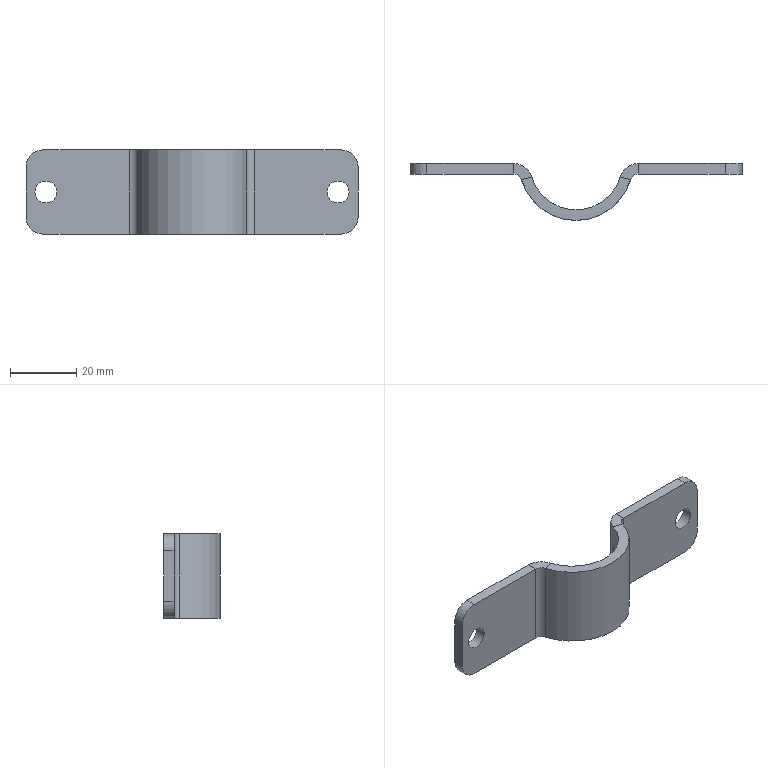Part | NX | features BREP 1 | 1 solid | 30 faces | box 100.076 x 17.145 x 25.4 mm | volume 8798 mm3 | plane 16 | cylinder 14 | commonest cylinder face diameters 6.604 x4 10.16 x4 4.978 x2 11.328 x2 27.94 x1 34.29 x1
STEP:
#1=CARTESIAN_POINT('',(-18.799,0.,12.7));
#2=VERTEX_POINT('',#1);
#3=CARTESIAN_POINT('',(-44.958,0.,12.7));
#4=VERTEX_POINT('',#3);
#5=CARTESIAN_POINT('',(-18.799,0.,12.7));
#6=DIRECTION('',(-1.,0.,0.));
#7=VECTOR('',#6,1000.);
#8=LINE('',#5,#7);
#9=EDGE_CURVE('',#2,#4,#8,.T.);
#10=ORIENTED_EDGE('',*,*,#9,.F.);
#11=CARTESIAN_POINT('',(-18.799,0.,-12.7));
#12=VERTEX_POINT('',#11);
#13=CARTESIAN_POINT('',(-18.799,0.,12.7));
#14=DIRECTION('',(0.,0.,-1.));
#15=VECTOR('',#14,1000.);
#16=LINE('',#13,#15);
#17=EDGE_CURVE('',#2,#12,#16,.T.);
#18=ORIENTED_EDGE('',*,*,#17,.T.);
#19=CARTESIAN_POINT('',(-44.958,0.,-12.7));
#20=VERTEX_POINT('',#19);
#21=CARTESIAN_POINT('',(-18.799,0.,-12.7));
#22=DIRECTION('',(-1.,0.,0.));
#23=VECTOR('',#22,1000.);
#24=LINE('',#21,#23);
#25=EDGE_CURVE('',#12,#20,#24,.T.);
#26=ORIENTED_EDGE('',*,*,#25,.T.);
#27=CARTESIAN_POINT('',(-50.038,0.,-7.62));
#28=VERTEX_POINT('',#27);
#29=CARTESIAN_POINT('',(-44.958,0.,-7.62));
#30=DIRECTION('',(0.,1.,0.));
#31=DIRECTION('',(0.,0.,-1.));
#32=AXIS2_PLACEMENT_3D('',#29,#30,#31);
#33=CIRCLE('',#32,5.08);
#34=EDGE_CURVE('',#20,#28,#33,.T.);
#35=ORIENTED_EDGE('',*,*,#34,.T.);
#36=CARTESIAN_POINT('',(-50.038,0.,7.62));
#37=VERTEX_POINT('',#36);
#38=CARTESIAN_POINT('',(-50.038,0.,7.62));
#39=DIRECTION('',(0.,0.,-1.));
#40=VECTOR('',#39,1000.);
#41=LINE('',#38,#40);
#42=EDGE_CURVE('',#37,#28,#41,.T.);
#43=ORIENTED_EDGE('',*,*,#42,.F.);
#44=CARTESIAN_POINT('',(-44.958,0.,7.62));
#45=DIRECTION('',(0.,1.,0.));
#46=DIRECTION('',(-1.,0.,0.));
#47=AXIS2_PLACEMENT_3D('',#44,#45,#46);
#48=CIRCLE('',#47,5.08);
#49=EDGE_CURVE('',#37,#4,#48,.T.);
#50=ORIENTED_EDGE('',*,*,#49,.T.);
#51=EDGE_LOOP('',(#10,#18,#26,#35,#43,#50));
#52=FACE_BOUND('',#51,.T.);
#53=CARTESIAN_POINT('',(-47.346,0.,0.));
#54=VERTEX_POINT('',#53);
#55=CARTESIAN_POINT('',(-40.742,0.,0.));
#56=VERTEX_POINT('',#55);
#57=CARTESIAN_POINT('',(-44.044,0.,0.));
#58=DIRECTION('',(0.,-1.,0.));
#59=DIRECTION('',(-1.,0.,0.));
#60=AXIS2_PLACEMENT_3D('',#57,#58,#59);
#61=CIRCLE('',#60,3.302);
#62=EDGE_CURVE('',#54,#56,#61,.T.);
#63=ORIENTED_EDGE('',*,*,#62,.T.);
#64=CARTESIAN_POINT('',(-44.044,0.,0.));
#65=DIRECTION('',(0.,-1.,0.));
#66=DIRECTION('',(1.,0.,0.));
#67=AXIS2_PLACEMENT_3D('',#64,#65,#66);
#68=CIRCLE('',#67,3.302);
#69=EDGE_CURVE('',#56,#54,#68,.T.);
#70=ORIENTED_EDGE('',*,*,#69,.T.);
#71=EDGE_LOOP('',(#63,#70));
#72=FACE_BOUND('',#71,.T.);
#73=CARTESIAN_POINT('',(-18.799,0.,12.7));
#74=DIRECTION('',(0.,1.,0.));
#75=DIRECTION('',(1.,0.,0.));
#76=AXIS2_PLACEMENT_3D('',#73,#74,#75);
#77=PLANE('',#76);
#78=ADVANCED_FACE('',(#52,#72),#77,.T.);
#79=CARTESIAN_POINT('',(-40.742,-3.175,0.));
#80=VERTEX_POINT('',#79);
#81=CARTESIAN_POINT('',(-40.742,0.,0.));
#82=DIRECTION('',(0.,-1.,0.));
#83=VECTOR('',#82,1000.);
#84=LINE('',#81,#83);
#85=EDGE_CURVE('',#80,#56,#84,.F.);
#86=ORIENTED_EDGE('',*,*,#85,.F.);
#87=CARTESIAN_POINT('',(-47.346,-3.175,0.));
#88=VERTEX_POINT('',#87);
#89=CARTESIAN_POINT('',(-44.044,-3.175,0.));
#90=DIRECTION('',(0.,-1.,0.));
#91=DIRECTION('',(1.,0.,0.));
#92=AXIS2_PLACEMENT_3D('',#89,#90,#91);
#93=CIRCLE('',#92,3.302);
#94=EDGE_CURVE('',#80,#88,#93,.T.);
#95=ORIENTED_EDGE('',*,*,#94,.T.);
#96=CARTESIAN_POINT('',(-47.346,0.,0.));
#97=DIRECTION('',(0.,-1.,0.));
#98=VECTOR('',#97,1000.);
#99=LINE('',#96,#98);
#100=EDGE_CURVE('',#88,#54,#99,.F.);
#101=ORIENTED_EDGE('',*,*,#100,.T.);
#102=ORIENTED_EDGE('',*,*,#69,.F.);
#103=EDGE_LOOP('',(#86,#95,#101,#102));
#104=FACE_BOUND('',#103,.T.);
#105=CARTESIAN_POINT('',(-44.044,-1.587,0.));
#106=DIRECTION('',(0.,-1.,0.));
#107=DIRECTION('',(1.,0.,0.));
#108=AXIS2_PLACEMENT_3D('',#105,#106,#107);
#109=CYLINDRICAL_SURFACE('',#108,3.302);
#110=ADVANCED_FACE('',(#104),#109,.F.);
#111=ORIENTED_EDGE('',*,*,#100,.F.);
#112=CARTESIAN_POINT('',(-44.044,-3.175,0.));
#113=DIRECTION('',(0.,-1.,0.));
#114=DIRECTION('',(-1.,0.,0.));
#115=AXIS2_PLACEMENT_3D('',#112,#113,#114);
#116=CIRCLE('',#115,3.302);
#117=EDGE_CURVE('',#88,#80,#116,.T.);
#118=ORIENTED_EDGE('',*,*,#117,.T.);
#119=ORIENTED_EDGE('',*,*,#85,.T.);
#120=ORIENTED_EDGE('',*,*,#62,.F.);
#121=EDGE_LOOP('',(#111,#118,#119,#120));
#122=FACE_BOUND('',#121,.T.);
#123=CARTESIAN_POINT('',(-44.044,-1.587,0.));
#124=DIRECTION('',(0.,-1.,0.));
#125=DIRECTION('',(-1.,0.,0.));
#126=AXIS2_PLACEMENT_3D('',#123,#124,#125);
#127=CYLINDRICAL_SURFACE('',#126,3.302);
#128=ADVANCED_FACE('',(#122),#127,.F.);
#129=CARTESIAN_POINT('',(-50.038,-3.175,7.62));
#130=VERTEX_POINT('',#129);
#131=CARTESIAN_POINT('',(-50.038,-3.175,-7.62));
#132=VERTEX_POINT('',#131);
#133=CARTESIAN_POINT('',(-50.038,-3.175,7.62));
#134=DIRECTION('',(0.,0.,-1.));
#135=VECTOR('',#134,1000.);
#136=LINE('',#133,#135);
#137=EDGE_CURVE('',#130,#132,#136,.T.);
#138=ORIENTED_EDGE('',*,*,#137,.T.);
#139=CARTESIAN_POINT('',(-44.958,-3.175,-12.7));
#140=VERTEX_POINT('',#139);
#141=CARTESIAN_POINT('',(-44.958,-3.175,-7.62));
#142=DIRECTION('',(0.,-1.,0.));
#143=DIRECTION('',(-1.,0.,0.));
#144=AXIS2_PLACEMENT_3D('',#141,#142,#143);
#145=CIRCLE('',#144,5.08);
#146=EDGE_CURVE('',#132,#140,#145,.T.);
#147=ORIENTED_EDGE('',*,*,#146,.T.);
#148=CARTESIAN_POINT('',(-18.799,-3.175,-12.7));
#149=VERTEX_POINT('',#148);
#150=CARTESIAN_POINT('',(-18.799,-3.175,-12.7));
#151=DIRECTION('',(-1.,0.,0.));
#152=VECTOR('',#151,1000.);
#153=LINE('',#150,#152);
#154=EDGE_CURVE('',#149,#140,#153,.T.);
#155=ORIENTED_EDGE('',*,*,#154,.F.);
#156=CARTESIAN_POINT('',(-18.799,-3.175,12.7));
#157=VERTEX_POINT('',#156);
#158=CARTESIAN_POINT('',(-18.799,-3.175,12.7));
#159=DIRECTION('',(0.,0.,-1.));
#160=VECTOR('',#159,1000.);
#161=LINE('',#158,#160);
#162=EDGE_CURVE('',#157,#149,#161,.T.);
#163=ORIENTED_EDGE('',*,*,#162,.F.);
#164=CARTESIAN_POINT('',(-44.958,-3.175,12.7));
#165=VERTEX_POINT('',#164);
#166=CARTESIAN_POINT('',(-18.799,-3.175,12.7));
#167=DIRECTION('',(-1.,0.,0.));
#168=VECTOR('',#167,1000.);
#169=LINE('',#166,#168);
#170=EDGE_CURVE('',#157,#165,#169,.T.);
#171=ORIENTED_EDGE('',*,*,#170,.T.);
#172=CARTESIAN_POINT('',(-44.958,-3.175,7.62));
#173=DIRECTION('',(0.,-1.,0.));
#174=DIRECTION('',(0.,0.,1.));
#175=AXIS2_PLACEMENT_3D('',#172,#173,#174);
#176=CIRCLE('',#175,5.08);
#177=EDGE_CURVE('',#165,#130,#176,.T.);
#178=ORIENTED_EDGE('',*,*,#177,.T.);
#179=EDGE_LOOP('',(#138,#147,#155,#163,#171,#178));
#180=FACE_BOUND('',#179,.T.);
#181=ORIENTED_EDGE('',*,*,#117,.F.);
#182=ORIENTED_EDGE('',*,*,#94,.F.);
#183=EDGE_LOOP('',(#181,#182));
#184=FACE_BOUND('',#183,.T.);
#185=CARTESIAN_POINT('',(-18.799,-3.175,12.7));
#186=DIRECTION('',(0.,1.,0.));
#187=DIRECTION('',(1.,0.,0.));
#188=AXIS2_PLACEMENT_3D('',#185,#186,#187);
#189=PLANE('',#188);
#190=ADVANCED_FACE('',(#180,#184),#189,.F.);
#191=ORIENTED_EDGE('',*,*,#177,.F.);
#192=CARTESIAN_POINT('',(-44.958,-3.175,12.7));
#193=DIRECTION('',(0.,1.,0.));
#194=VECTOR('',#193,1000.);
#195=LINE('',#192,#194);
#196=EDGE_CURVE('',#165,#4,#195,.T.);
#197=ORIENTED_EDGE('',*,*,#196,.T.);
#198=ORIENTED_EDGE('',*,*,#49,.F.);
#199=CARTESIAN_POINT('',(-50.038,-3.175,7.62));
#200=DIRECTION('',(0.,1.,0.));
#201=VECTOR('',#200,1000.);
#202=LINE('',#199,#201);
#203=EDGE_CURVE('',#130,#37,#202,.T.);
#204=ORIENTED_EDGE('',*,*,#203,.F.);
#205=EDGE_LOOP('',(#191,#197,#198,#204));
#206=FACE_BOUND('',#205,.T.);
#207=CARTESIAN_POINT('',(-44.958,-3.317,7.62));
#208=DIRECTION('',(0.,1.,0.));
#209=DIRECTION('',(-1.,0.,0.));
#210=AXIS2_PLACEMENT_3D('',#207,#208,#209);
#211=CYLINDRICAL_SURFACE('',#210,5.08);
#212=ADVANCED_FACE('',(#206),#211,.T.);
#213=ORIENTED_EDGE('',*,*,#42,.T.);
#214=CARTESIAN_POINT('',(-50.038,-3.175,-7.62));
#215=DIRECTION('',(0.,1.,0.));
#216=VECTOR('',#215,1000.);
#217=LINE('',#214,#216);
#218=EDGE_CURVE('',#132,#28,#217,.T.);
#219=ORIENTED_EDGE('',*,*,#218,.F.);
#220=ORIENTED_EDGE('',*,*,#137,.F.);
#221=ORIENTED_EDGE('',*,*,#203,.T.);
#222=EDGE_LOOP('',(#213,#219,#220,#221));
#223=FACE_BOUND('',#222,.T.);
#224=CARTESIAN_POINT('',(-50.038,-1.587,0.));
#225=DIRECTION('',(1.,0.,0.));
#226=DIRECTION('',(0.,1.,0.));
#227=AXIS2_PLACEMENT_3D('',#224,#225,#226);
#228=PLANE('',#227);
#229=ADVANCED_FACE('',(#223),#228,.F.);
#230=ORIENTED_EDGE('',*,*,#146,.F.);
#231=ORIENTED_EDGE('',*,*,#218,.T.);
#232=ORIENTED_EDGE('',*,*,#34,.F.);
#233=CARTESIAN_POINT('',(-44.958,-3.175,-12.7));
#234=DIRECTION('',(0.,1.,0.));
#235=VECTOR('',#234,1000.);
#236=LINE('',#233,#235);
#237=EDGE_CURVE('',#140,#20,#236,.T.);
#238=ORIENTED_EDGE('',*,*,#237,.F.);
#239=EDGE_LOOP('',(#230,#231,#232,#238));
#240=FACE_BOUND('',#239,.T.);
#241=CARTESIAN_POINT('',(-44.958,-3.317,-7.62));
#242=DIRECTION('',(0.,1.,0.));
#243=DIRECTION('',(0.,0.,-1.));
#244=AXIS2_PLACEMENT_3D('',#241,#242,#243);
#245=CYLINDRICAL_SURFACE('',#244,5.08);
#246=ADVANCED_FACE('',(#240),#245,.T.);
#247=ORIENTED_EDGE('',*,*,#25,.F.);
#248=CARTESIAN_POINT('',(-18.799,0.,-12.7));
#249=DIRECTION('',(0.,-1.,0.));
#250=VECTOR('',#249,1000.);
#251=LINE('',#248,#250);
#252=EDGE_CURVE('',#12,#149,#251,.T.);
#253=ORIENTED_EDGE('',*,*,#252,.T.);
#254=ORIENTED_EDGE('',*,*,#154,.T.);
#255=ORIENTED_EDGE('',*,*,#237,.T.);
#256=EDGE_LOOP('',(#247,#253,#254,#255));
#257=FACE_BOUND('',#256,.T.);
#258=CARTESIAN_POINT('',(-34.419,-1.587,-12.7));
#259=DIRECTION('',(0.,0.,-1.));
#260=DIRECTION('',(0.,-1.,0.));
#261=AXIS2_PLACEMENT_3D('',#258,#259,#260);
#262=PLANE('',#261);
#263=ADVANCED_FACE('',(#257),#262,.T.);
#264=CARTESIAN_POINT('',(-13.376,-4.03,-12.7));
#265=VERTEX_POINT('',#264);
#266=CARTESIAN_POINT('',(-16.416,-4.946,-12.7));
#267=VERTEX_POINT('',#266);
#268=CARTESIAN_POINT('',(-13.376,-4.03,-12.7));
#269=DIRECTION('',(-0.9575,-0.2885,0.));
#270=VECTOR('',#269,1000.);
#271=LINE('',#268,#270);
#272=EDGE_CURVE('',#265,#267,#271,.T.);
#273=ORIENTED_EDGE('',*,*,#272,.T.);
#274=CARTESIAN_POINT('',(-18.799,-5.664,-12.7));
#275=DIRECTION('',(0.,0.,1.));
#276=DIRECTION('',(0.9575,0.2885,0.));
#277=AXIS2_PLACEMENT_3D('',#274,#275,#276);
#278=CIRCLE('',#277,2.489);
#279=EDGE_CURVE('',#267,#149,#278,.T.);
#280=ORIENTED_EDGE('',*,*,#279,.T.);
#281=ORIENTED_EDGE('',*,*,#252,.F.);
#282=CARTESIAN_POINT('',(-18.799,-5.664,-12.7));
#283=DIRECTION('',(0.,0.,1.));
#284=DIRECTION('',(0.9575,0.2885,0.));
#285=AXIS2_PLACEMENT_3D('',#282,#283,#284);
#286=CIRCLE('',#285,5.664);
#287=EDGE_CURVE('',#265,#12,#286,.T.);
#288=ORIENTED_EDGE('',*,*,#287,.F.);
#289=EDGE_LOOP('',(#273,#280,#281,#288));
#290=FACE_BOUND('',#289,.T.);
#291=CARTESIAN_POINT('',(-16.368,-2.392,-12.7));
#292=DIRECTION('',(0.,0.,-1.));
#293=DIRECTION('',(0.,-1.,0.));
#294=AXIS2_PLACEMENT_3D('',#291,#292,#293);
#295=PLANE('',#294);
#296=ADVANCED_FACE('',(#290),#295,.T.);
#297=CARTESIAN_POINT('',(-13.376,-4.03,12.7));
#298=VERTEX_POINT('',#297);
#299=CARTESIAN_POINT('',(-13.376,-4.03,12.7));
#300=DIRECTION('',(0.,0.,-1.));
#301=VECTOR('',#300,1000.);
#302=LINE('',#299,#301);
#303=EDGE_CURVE('',#298,#265,#302,.T.);
#304=ORIENTED_EDGE('',*,*,#303,.T.);
#305=ORIENTED_EDGE('',*,*,#287,.T.);
#306=ORIENTED_EDGE('',*,*,#17,.F.);
#307=CARTESIAN_POINT('',(-18.799,-5.664,12.7));
#308=DIRECTION('',(0.,0.,1.));
#309=DIRECTION('',(0.9575,0.2885,0.));
#310=AXIS2_PLACEMENT_3D('',#307,#308,#309);
#311=CIRCLE('',#310,5.664);
#312=EDGE_CURVE('',#298,#2,#311,.T.);
#313=ORIENTED_EDGE('',*,*,#312,.F.);
#314=EDGE_LOOP('',(#304,#305,#306,#313));
#315=FACE_BOUND('',#314,.T.);
#316=CARTESIAN_POINT('',(-18.799,-5.664,12.7));
#317=DIRECTION('',(0.,0.,1.));
#318=DIRECTION('',(1.,0.,0.));
#319=AXIS2_PLACEMENT_3D('',#316,#317,#318);
#320=CYLINDRICAL_SURFACE('',#319,5.664);
#321=ADVANCED_FACE('',(#315),#320,.T.);
#322=CARTESIAN_POINT('',(-18.799,0.,12.7));
#323=DIRECTION('',(0.,-1.,0.));
#324=VECTOR('',#323,1000.);
#325=LINE('',#322,#324);
#326=EDGE_CURVE('',#2,#157,#325,.T.);
#327=ORIENTED_EDGE('',*,*,#326,.T.);
#328=CARTESIAN_POINT('',(-16.416,-4.946,12.7));
#329=VERTEX_POINT('',#328);
#330=CARTESIAN_POINT('',(-18.799,-5.664,12.7));
#331=DIRECTION('',(0.,0.,1.));
#332=DIRECTION('',(0.9575,0.2885,0.));
#333=AXIS2_PLACEMENT_3D('',#330,#331,#332);
#334=CIRCLE('',#333,2.489);
#335=EDGE_CURVE('',#329,#157,#334,.T.);
#336=ORIENTED_EDGE('',*,*,#335,.F.);
#337=CARTESIAN_POINT('',(-13.376,-4.03,12.7));
#338=DIRECTION('',(-0.9575,-0.2885,0.));
#339=VECTOR('',#338,1000.);
#340=LINE('',#337,#339);
#341=EDGE_CURVE('',#298,#329,#340,.T.);
#342=ORIENTED_EDGE('',*,*,#341,.F.);
#343=ORIENTED_EDGE('',*,*,#312,.T.);
#344=EDGE_LOOP('',(#327,#336,#342,#343));
#345=FACE_BOUND('',#344,.T.);
#346=CARTESIAN_POINT('',(-16.368,-2.392,12.7));
#347=DIRECTION('',(0.,0.,-1.));
#348=DIRECTION('',(0.,-1.,0.));
#349=AXIS2_PLACEMENT_3D('',#346,#347,#348);
#350=PLANE('',#349);
#351=ADVANCED_FACE('',(#345),#350,.F.);
#352=ORIENTED_EDGE('',*,*,#341,.T.);
#353=CARTESIAN_POINT('',(16.416,-4.946,12.7));
#354=VERTEX_POINT('',#353);
#355=CARTESIAN_POINT('',(0.,0.,12.7));
#356=DIRECTION('',(0.,0.,-1.));
#357=DIRECTION('',(0.9575,-0.2885,0.));
#358=AXIS2_PLACEMENT_3D('',#355,#356,#357);
#359=CIRCLE('',#358,17.145);
#360=EDGE_CURVE('',#354,#329,#359,.T.);
#361=ORIENTED_EDGE('',*,*,#360,.F.);
#362=CARTESIAN_POINT('',(13.376,-4.03,12.7));
#363=VERTEX_POINT('',#362);
#364=CARTESIAN_POINT('',(13.376,-4.03,12.7));
#365=DIRECTION('',(0.9575,-0.2885,0.));
#366=VECTOR('',#365,1000.);
#367=LINE('',#364,#366);
#368=EDGE_CURVE('',#363,#354,#367,.T.);
#369=ORIENTED_EDGE('',*,*,#368,.F.);
#370=CARTESIAN_POINT('',(0.,0.,12.7));
#371=DIRECTION('',(0.,0.,-1.));
#372=DIRECTION('',(0.9575,-0.2885,0.));
#373=AXIS2_PLACEMENT_3D('',#370,#371,#372);
#374=CIRCLE('',#373,13.97);
#375=EDGE_CURVE('',#363,#298,#374,.T.);
#376=ORIENTED_EDGE('',*,*,#375,.T.);
#377=EDGE_LOOP('',(#352,#361,#369,#376));
#378=FACE_BOUND('',#377,.T.);
#379=CARTESIAN_POINT('',(0.,-15.557,12.7));
#380=DIRECTION('',(0.,0.,-1.));
#381=DIRECTION('',(0.,-1.,0.));
#382=AXIS2_PLACEMENT_3D('',#379,#380,#381);
#383=PLANE('',#382);
#384=ADVANCED_FACE('',(#378),#383,.F.);
#385=CARTESIAN_POINT('',(13.376,-4.03,-12.7));
#386=VERTEX_POINT('',#385);
#387=CARTESIAN_POINT('',(13.376,-4.03,12.7));
#388=DIRECTION('',(0.,0.,-1.));
#389=VECTOR('',#388,1000.);
#390=LINE('',#387,#389);
#391=EDGE_CURVE('',#363,#386,#390,.T.);
#392=ORIENTED_EDGE('',*,*,#391,.T.);
#393=CARTESIAN_POINT('',(0.,0.,-12.7));
#394=DIRECTION('',(0.,0.,-1.));
#395=DIRECTION('',(0.9575,-0.2885,0.));
#396=AXIS2_PLACEMENT_3D('',#393,#394,#395);
#397=CIRCLE('',#396,13.97);
#398=EDGE_CURVE('',#386,#265,#397,.T.);
#399=ORIENTED_EDGE('',*,*,#398,.T.);
#400=ORIENTED_EDGE('',*,*,#303,.F.);
#401=ORIENTED_EDGE('',*,*,#375,.F.);
#402=EDGE_LOOP('',(#392,#399,#400,#401));
#403=FACE_BOUND('',#402,.T.);
#404=CARTESIAN_POINT('',(0.,0.,12.7));
#405=DIRECTION('',(0.,0.,1.));
#406=DIRECTION('',(1.,0.,0.));
#407=AXIS2_PLACEMENT_3D('',#404,#405,#406);
#408=CYLINDRICAL_SURFACE('',#407,13.97);
#409=ADVANCED_FACE('',(#403),#408,.F.);
#410=CARTESIAN_POINT('',(16.416,-4.946,-12.7));
#411=VERTEX_POINT('',#410);
#412=CARTESIAN_POINT('',(13.376,-4.03,-12.7));
#413=DIRECTION('',(0.9575,-0.2885,0.));
#414=VECTOR('',#413,1000.);
#415=LINE('',#412,#414);
#416=EDGE_CURVE('',#386,#411,#415,.T.);
#417=ORIENTED_EDGE('',*,*,#416,.T.);
#418=CARTESIAN_POINT('',(0.,0.,-12.7));
#419=DIRECTION('',(0.,0.,-1.));
#420=DIRECTION('',(0.9575,-0.2885,0.));
#421=AXIS2_PLACEMENT_3D('',#418,#419,#420);
#422=CIRCLE('',#421,17.145);
#423=EDGE_CURVE('',#411,#267,#422,.T.);
#424=ORIENTED_EDGE('',*,*,#423,.T.);
#425=ORIENTED_EDGE('',*,*,#272,.F.);
#426=ORIENTED_EDGE('',*,*,#398,.F.);
#427=EDGE_LOOP('',(#417,#424,#425,#426));
#428=FACE_BOUND('',#427,.T.);
#429=CARTESIAN_POINT('',(0.,-15.557,-12.7));
#430=DIRECTION('',(0.,0.,-1.));
#431=DIRECTION('',(0.,-1.,0.));
#432=AXIS2_PLACEMENT_3D('',#429,#430,#431);
#433=PLANE('',#432);
#434=ADVANCED_FACE('',(#428),#433,.T.);
#435=CARTESIAN_POINT('',(-16.416,-4.946,12.7));
#436=DIRECTION('',(0.,0.,-1.));
#437=VECTOR('',#436,1000.);
#438=LINE('',#435,#437);
#439=EDGE_CURVE('',#329,#267,#438,.T.);
#440=ORIENTED_EDGE('',*,*,#439,.T.);
#441=ORIENTED_EDGE('',*,*,#423,.F.);
#442=CARTESIAN_POINT('',(16.416,-4.946,12.7));
#443=DIRECTION('',(0.,0.,-1.));
#444=VECTOR('',#443,1000.);
#445=LINE('',#442,#444);
#446=EDGE_CURVE('',#354,#411,#445,.T.);
#447=ORIENTED_EDGE('',*,*,#446,.F.);
#448=ORIENTED_EDGE('',*,*,#360,.T.);
#449=EDGE_LOOP('',(#440,#441,#447,#448));
#450=FACE_BOUND('',#449,.T.);
#451=CARTESIAN_POINT('',(0.,0.,12.7));
#452=DIRECTION('',(0.,0.,1.));
#453=DIRECTION('',(1.,0.,0.));
#454=AXIS2_PLACEMENT_3D('',#451,#452,#453);
#455=CYLINDRICAL_SURFACE('',#454,17.145);
#456=ADVANCED_FACE('',(#450),#455,.T.);
#457=ORIENTED_EDGE('',*,*,#446,.T.);
#458=CARTESIAN_POINT('',(18.799,-3.175,-12.7));
#459=VERTEX_POINT('',#458);
#460=CARTESIAN_POINT('',(18.799,-5.664,-12.7));
#461=DIRECTION('',(0.,0.,1.));
#462=DIRECTION('',(0.,1.,0.));
#463=AXIS2_PLACEMENT_3D('',#460,#461,#462);
#464=CIRCLE('',#463,2.489);
#465=EDGE_CURVE('',#459,#411,#464,.T.);
#466=ORIENTED_EDGE('',*,*,#465,.F.);
#467=CARTESIAN_POINT('',(18.799,-3.175,12.7));
#468=VERTEX_POINT('',#467);
#469=CARTESIAN_POINT('',(18.799,-3.175,12.7));
#470=DIRECTION('',(0.,0.,-1.));
#471=VECTOR('',#470,1000.);
#472=LINE('',#469,#471);
#473=EDGE_CURVE('',#468,#459,#472,.T.);
#474=ORIENTED_EDGE('',*,*,#473,.F.);
#475=CARTESIAN_POINT('',(18.799,-5.664,12.7));
#476=DIRECTION('',(0.,0.,1.));
#477=DIRECTION('',(0.,1.,0.));
#478=AXIS2_PLACEMENT_3D('',#475,#476,#477);
#479=CIRCLE('',#478,2.489);
#480=EDGE_CURVE('',#468,#354,#479,.T.);
#481=ORIENTED_EDGE('',*,*,#480,.T.);
#482=EDGE_LOOP('',(#457,#466,#474,#481));
#483=FACE_BOUND('',#482,.T.);
#484=CARTESIAN_POINT('',(18.799,-5.664,12.7));
#485=DIRECTION('',(0.,0.,1.));
#486=DIRECTION('',(1.,0.,0.));
#487=AXIS2_PLACEMENT_3D('',#484,#485,#486);
#488=CYLINDRICAL_SURFACE('',#487,2.489);
#489=ADVANCED_FACE('',(#483),#488,.F.);
#490=ORIENTED_EDGE('',*,*,#368,.T.);
#491=ORIENTED_EDGE('',*,*,#480,.F.);
#492=CARTESIAN_POINT('',(18.799,0.,12.7));
#493=VERTEX_POINT('',#492);
#494=CARTESIAN_POINT('',(18.799,0.,12.7));
#495=DIRECTION('',(0.,-1.,0.));
#496=VECTOR('',#495,1000.);
#497=LINE('',#494,#496);
#498=EDGE_CURVE('',#493,#468,#497,.T.);
#499=ORIENTED_EDGE('',*,*,#498,.F.);
#500=CARTESIAN_POINT('',(18.799,-5.664,12.7));
#501=DIRECTION('',(0.,0.,1.));
#502=DIRECTION('',(0.,1.,0.));
#503=AXIS2_PLACEMENT_3D('',#500,#501,#502);
#504=CIRCLE('',#503,5.664);
#505=EDGE_CURVE('',#493,#363,#504,.T.);
#506=ORIENTED_EDGE('',*,*,#505,.T.);
#507=EDGE_LOOP('',(#490,#491,#499,#506));
#508=FACE_BOUND('',#507,.T.);
#509=CARTESIAN_POINT('',(16.368,-2.392,12.7));
#510=DIRECTION('',(0.,0.,-1.));
#511=DIRECTION('',(0.,-1.,0.));
#512=AXIS2_PLACEMENT_3D('',#509,#510,#511);
#513=PLANE('',#512);
#514=ADVANCED_FACE('',(#508),#513,.F.);
#515=CARTESIAN_POINT('',(18.799,0.,-12.7));
#516=VERTEX_POINT('',#515);
#517=CARTESIAN_POINT('',(18.799,0.,12.7));
#518=DIRECTION('',(0.,0.,-1.));
#519=VECTOR('',#518,1000.);
#520=LINE('',#517,#519);
#521=EDGE_CURVE('',#493,#516,#520,.T.);
#522=ORIENTED_EDGE('',*,*,#521,.T.);
#523=CARTESIAN_POINT('',(18.799,-5.664,-12.7));
#524=DIRECTION('',(0.,0.,1.));
#525=DIRECTION('',(0.,1.,0.));
#526=AXIS2_PLACEMENT_3D('',#523,#524,#525);
#527=CIRCLE('',#526,5.664);
#528=EDGE_CURVE('',#516,#386,#527,.T.);
#529=ORIENTED_EDGE('',*,*,#528,.T.);
#530=ORIENTED_EDGE('',*,*,#391,.F.);
#531=ORIENTED_EDGE('',*,*,#505,.F.);
#532=EDGE_LOOP('',(#522,#529,#530,#531));
#533=FACE_BOUND('',#532,.T.);
#534=CARTESIAN_POINT('',(18.799,-5.664,12.7));
#535=DIRECTION('',(0.,0.,1.));
#536=DIRECTION('',(1.,0.,0.));
#537=AXIS2_PLACEMENT_3D('',#534,#535,#536);
#538=CYLINDRICAL_SURFACE('',#537,5.664);
#539=ADVANCED_FACE('',(#533),#538,.T.);
#540=CARTESIAN_POINT('',(18.799,0.,-12.7));
#541=DIRECTION('',(0.,-1.,0.));
#542=VECTOR('',#541,1000.);
#543=LINE('',#540,#542);
#544=EDGE_CURVE('',#516,#459,#543,.T.);
#545=ORIENTED_EDGE('',*,*,#544,.T.);
#546=ORIENTED_EDGE('',*,*,#465,.T.);
#547=ORIENTED_EDGE('',*,*,#416,.F.);
#548=ORIENTED_EDGE('',*,*,#528,.F.);
#549=EDGE_LOOP('',(#545,#546,#547,#548));
#550=FACE_BOUND('',#549,.T.);
#551=CARTESIAN_POINT('',(16.368,-2.392,-12.7));
#552=DIRECTION('',(0.,0.,-1.));
#553=DIRECTION('',(0.,-1.,0.));
#554=AXIS2_PLACEMENT_3D('',#551,#552,#553);
#555=PLANE('',#554);
#556=ADVANCED_FACE('',(#550),#555,.T.);
#557=CARTESIAN_POINT('',(44.958,-3.175,-12.7));
#558=VERTEX_POINT('',#557);
#559=CARTESIAN_POINT('',(44.958,-3.175,-12.7));
#560=DIRECTION('',(-1.,0.,0.));
#561=VECTOR('',#560,1000.);
#562=LINE('',#559,#561);
#563=EDGE_CURVE('',#558,#459,#562,.T.);
#564=ORIENTED_EDGE('',*,*,#563,.T.);
#565=ORIENTED_EDGE('',*,*,#544,.F.);
#566=CARTESIAN_POINT('',(44.958,0.,-12.7));
#567=VERTEX_POINT('',#566);
#568=CARTESIAN_POINT('',(44.958,0.,-12.7));
#569=DIRECTION('',(-1.,0.,0.));
#570=VECTOR('',#569,1000.);
#571=LINE('',#568,#570);
#572=EDGE_CURVE('',#567,#516,#571,.T.);
#573=ORIENTED_EDGE('',*,*,#572,.F.);
#574=CARTESIAN_POINT('',(44.958,-3.175,-12.7));
#575=DIRECTION('',(0.,1.,0.));
#576=VECTOR('',#575,1000.);
#577=LINE('',#574,#576);
#578=EDGE_CURVE('',#558,#567,#577,.T.);
#579=ORIENTED_EDGE('',*,*,#578,.F.);
#580=EDGE_LOOP('',(#564,#565,#573,#579));
#581=FACE_BOUND('',#580,.T.);
#582=CARTESIAN_POINT('',(34.419,-1.587,-12.7));
#583=DIRECTION('',(0.,0.,-1.));
#584=DIRECTION('',(0.,-1.,0.));
#585=AXIS2_PLACEMENT_3D('',#582,#583,#584);
#586=PLANE('',#585);
#587=ADVANCED_FACE('',(#581),#586,.T.);
#588=CARTESIAN_POINT('',(50.038,-3.175,-7.62));
#589=VERTEX_POINT('',#588);
#590=CARTESIAN_POINT('',(44.958,-3.175,-7.62));
#591=DIRECTION('',(0.,-1.,0.));
#592=DIRECTION('',(0.,0.,-1.));
#593=AXIS2_PLACEMENT_3D('',#590,#591,#592);
#594=CIRCLE('',#593,5.08);
#595=EDGE_CURVE('',#558,#589,#594,.T.);
#596=ORIENTED_EDGE('',*,*,#595,.F.);
#597=ORIENTED_EDGE('',*,*,#578,.T.);
#598=CARTESIAN_POINT('',(50.038,0.,-7.62));
#599=VERTEX_POINT('',#598);
#600=CARTESIAN_POINT('',(44.958,0.,-7.62));
#601=DIRECTION('',(0.,1.,0.));
#602=DIRECTION('',(1.,0.,0.));
#603=AXIS2_PLACEMENT_3D('',#600,#601,#602);
#604=CIRCLE('',#603,5.08);
#605=EDGE_CURVE('',#599,#567,#604,.T.);
#606=ORIENTED_EDGE('',*,*,#605,.F.);
#607=CARTESIAN_POINT('',(50.038,-3.175,-7.62));
#608=DIRECTION('',(0.,1.,0.));
#609=VECTOR('',#608,1000.);
#610=LINE('',#607,#609);
#611=EDGE_CURVE('',#589,#599,#610,.T.);
#612=ORIENTED_EDGE('',*,*,#611,.F.);
#613=EDGE_LOOP('',(#596,#597,#606,#612));
#614=FACE_BOUND('',#613,.T.);
#615=CARTESIAN_POINT('',(44.958,-3.317,-7.62));
#616=DIRECTION('',(0.,1.,0.));
#617=DIRECTION('',(1.,0.,0.));
#618=AXIS2_PLACEMENT_3D('',#615,#616,#617);
#619=CYLINDRICAL_SURFACE('',#618,5.08);
#620=ADVANCED_FACE('',(#614),#619,.T.);
#621=CARTESIAN_POINT('',(50.038,-3.175,7.62));
#622=VERTEX_POINT('',#621);
#623=CARTESIAN_POINT('',(50.038,-3.175,7.62));
#624=DIRECTION('',(0.,0.,-1.));
#625=VECTOR('',#624,1000.);
#626=LINE('',#623,#625);
#627=EDGE_CURVE('',#622,#589,#626,.T.);
#628=ORIENTED_EDGE('',*,*,#627,.T.);
#629=ORIENTED_EDGE('',*,*,#611,.T.);
#630=CARTESIAN_POINT('',(50.038,0.,7.62));
#631=VERTEX_POINT('',#630);
#632=CARTESIAN_POINT('',(50.038,0.,7.62));
#633=DIRECTION('',(0.,0.,-1.));
#634=VECTOR('',#633,1000.);
#635=LINE('',#632,#634);
#636=EDGE_CURVE('',#631,#599,#635,.T.);
#637=ORIENTED_EDGE('',*,*,#636,.F.);
#638=CARTESIAN_POINT('',(50.038,-3.175,7.62));
#639=DIRECTION('',(0.,1.,0.));
#640=VECTOR('',#639,1000.);
#641=LINE('',#638,#640);
#642=EDGE_CURVE('',#622,#631,#641,.T.);
#643=ORIENTED_EDGE('',*,*,#642,.F.);
#644=EDGE_LOOP('',(#628,#629,#637,#643));
#645=FACE_BOUND('',#644,.T.);
#646=CARTESIAN_POINT('',(50.038,-1.587,0.));
#647=DIRECTION('',(1.,0.,0.));
#648=DIRECTION('',(0.,1.,0.));
#649=AXIS2_PLACEMENT_3D('',#646,#647,#648);
#650=PLANE('',#649);
#651=ADVANCED_FACE('',(#645),#650,.T.);
#652=CARTESIAN_POINT('',(44.958,-3.175,12.7));
#653=VERTEX_POINT('',#652);
#654=CARTESIAN_POINT('',(44.958,-3.175,7.62));
#655=DIRECTION('',(0.,-1.,0.));
#656=DIRECTION('',(1.,0.,0.));
#657=AXIS2_PLACEMENT_3D('',#654,#655,#656);
#658=CIRCLE('',#657,5.08);
#659=EDGE_CURVE('',#622,#653,#658,.T.);
#660=ORIENTED_EDGE('',*,*,#659,.F.);
#661=ORIENTED_EDGE('',*,*,#642,.T.);
#662=CARTESIAN_POINT('',(44.958,0.,12.7));
#663=VERTEX_POINT('',#662);
#664=CARTESIAN_POINT('',(44.958,0.,7.62));
#665=DIRECTION('',(0.,1.,0.));
#666=DIRECTION('',(0.,0.,1.));
#667=AXIS2_PLACEMENT_3D('',#664,#665,#666);
#668=CIRCLE('',#667,5.08);
#669=EDGE_CURVE('',#663,#631,#668,.T.);
#670=ORIENTED_EDGE('',*,*,#669,.F.);
#671=CARTESIAN_POINT('',(44.958,-3.175,12.7));
#672=DIRECTION('',(0.,1.,0.));
#673=VECTOR('',#672,1000.);
#674=LINE('',#671,#673);
#675=EDGE_CURVE('',#653,#663,#674,.T.);
#676=ORIENTED_EDGE('',*,*,#675,.F.);
#677=EDGE_LOOP('',(#660,#661,#670,#676));
#678=FACE_BOUND('',#677,.T.);
#679=CARTESIAN_POINT('',(44.958,-3.317,7.62));
#680=DIRECTION('',(0.,1.,0.));
#681=DIRECTION('',(0.,0.,1.));
#682=AXIS2_PLACEMENT_3D('',#679,#680,#681);
#683=CYLINDRICAL_SURFACE('',#682,5.08);
#684=ADVANCED_FACE('',(#678),#683,.T.);
#685=CARTESIAN_POINT('',(44.958,0.,12.7));
#686=DIRECTION('',(-1.,0.,0.));
#687=VECTOR('',#686,1000.);
#688=LINE('',#685,#687);
#689=EDGE_CURVE('',#663,#493,#688,.T.);
#690=ORIENTED_EDGE('',*,*,#689,.T.);
#691=ORIENTED_EDGE('',*,*,#498,.T.);
#692=CARTESIAN_POINT('',(44.958,-3.175,12.7));
#693=DIRECTION('',(-1.,0.,0.));
#694=VECTOR('',#693,1000.);
#695=LINE('',#692,#694);
#696=EDGE_CURVE('',#653,#468,#695,.T.);
#697=ORIENTED_EDGE('',*,*,#696,.F.);
#698=ORIENTED_EDGE('',*,*,#675,.T.);
#699=EDGE_LOOP('',(#690,#691,#697,#698));
#700=FACE_BOUND('',#699,.T.);
#701=CARTESIAN_POINT('',(34.419,-1.587,12.7));
#702=DIRECTION('',(0.,0.,-1.));
#703=DIRECTION('',(0.,-1.,0.));
#704=AXIS2_PLACEMENT_3D('',#701,#702,#703);
#705=PLANE('',#704);
#706=ADVANCED_FACE('',(#700),#705,.F.);
#707=ORIENTED_EDGE('',*,*,#696,.T.);
#708=ORIENTED_EDGE('',*,*,#473,.T.);
#709=ORIENTED_EDGE('',*,*,#563,.F.);
#710=ORIENTED_EDGE('',*,*,#595,.T.);
#711=ORIENTED_EDGE('',*,*,#627,.F.);
#712=ORIENTED_EDGE('',*,*,#659,.T.);
#713=EDGE_LOOP('',(#707,#708,#709,#710,#711,#712));
#714=FACE_BOUND('',#713,.T.);
#715=CARTESIAN_POINT('',(47.346,-3.175,0.));
#716=VERTEX_POINT('',#715);
#717=CARTESIAN_POINT('',(40.742,-3.175,0.));
#718=VERTEX_POINT('',#717);
#719=CARTESIAN_POINT('',(44.044,-3.175,0.));
#720=DIRECTION('',(0.,1.,0.));
#721=DIRECTION('',(1.,0.,0.));
#722=AXIS2_PLACEMENT_3D('',#719,#720,#721);
#723=CIRCLE('',#722,3.302);
#724=EDGE_CURVE('',#716,#718,#723,.T.);
#725=ORIENTED_EDGE('',*,*,#724,.T.);
#726=CARTESIAN_POINT('',(44.044,-3.175,0.));
#727=DIRECTION('',(0.,1.,0.));
#728=DIRECTION('',(-1.,0.,0.));
#729=AXIS2_PLACEMENT_3D('',#726,#727,#728);
#730=CIRCLE('',#729,3.302);
#731=EDGE_CURVE('',#718,#716,#730,.T.);
#732=ORIENTED_EDGE('',*,*,#731,.T.);
#733=EDGE_LOOP('',(#725,#732));
#734=FACE_BOUND('',#733,.T.);
#735=CARTESIAN_POINT('',(50.038,-3.175,12.7));
#736=DIRECTION('',(0.,1.,0.));
#737=DIRECTION('',(1.,0.,0.));
#738=AXIS2_PLACEMENT_3D('',#735,#736,#737);
#739=PLANE('',#738);
#740=ADVANCED_FACE('',(#714,#734),#739,.F.);
#741=CARTESIAN_POINT('',(47.346,0.,0.));
#742=VERTEX_POINT('',#741);
#743=CARTESIAN_POINT('',(47.346,0.,0.));
#744=DIRECTION('',(0.,-1.,0.));
#745=VECTOR('',#744,1000.);
#746=LINE('',#743,#745);
#747=EDGE_CURVE('',#716,#742,#746,.F.);
#748=ORIENTED_EDGE('',*,*,#747,.F.);
#749=ORIENTED_EDGE('',*,*,#731,.F.);
#750=CARTESIAN_POINT('',(40.742,0.,0.));
#751=VERTEX_POINT('',#750);
#752=CARTESIAN_POINT('',(40.742,0.,0.));
#753=DIRECTION('',(0.,-1.,0.));
#754=VECTOR('',#753,1000.);
#755=LINE('',#752,#754);
#756=EDGE_CURVE('',#718,#751,#755,.F.);
#757=ORIENTED_EDGE('',*,*,#756,.T.);
#758=CARTESIAN_POINT('',(44.044,0.,0.));
#759=DIRECTION('',(0.,1.,0.));
#760=DIRECTION('',(-1.,0.,0.));
#761=AXIS2_PLACEMENT_3D('',#758,#759,#760);
#762=CIRCLE('',#761,3.302);
#763=EDGE_CURVE('',#751,#742,#762,.T.);
#764=ORIENTED_EDGE('',*,*,#763,.T.);
#765=EDGE_LOOP('',(#748,#749,#757,#764));
#766=FACE_BOUND('',#765,.T.);
#767=CARTESIAN_POINT('',(44.044,-1.587,0.));
#768=DIRECTION('',(0.,1.,0.));
#769=DIRECTION('',(-1.,0.,0.));
#770=AXIS2_PLACEMENT_3D('',#767,#768,#769);
#771=CYLINDRICAL_SURFACE('',#770,3.302);
#772=ADVANCED_FACE('',(#766),#771,.F.);
#773=ORIENTED_EDGE('',*,*,#636,.T.);
#774=ORIENTED_EDGE('',*,*,#605,.T.);
#775=ORIENTED_EDGE('',*,*,#572,.T.);
#776=ORIENTED_EDGE('',*,*,#521,.F.);
#777=ORIENTED_EDGE('',*,*,#689,.F.);
#778=ORIENTED_EDGE('',*,*,#669,.T.);
#779=EDGE_LOOP('',(#773,#774,#775,#776,#777,#778));
#780=FACE_BOUND('',#779,.T.);
#781=CARTESIAN_POINT('',(44.044,0.,0.));
#782=DIRECTION('',(0.,1.,0.));
#783=DIRECTION('',(1.,0.,0.));
#784=AXIS2_PLACEMENT_3D('',#781,#782,#783);
#785=CIRCLE('',#784,3.302);
#786=EDGE_CURVE('',#742,#751,#785,.T.);
#787=ORIENTED_EDGE('',*,*,#786,.F.);
#788=ORIENTED_EDGE('',*,*,#763,.F.);
#789=EDGE_LOOP('',(#787,#788));
#790=FACE_BOUND('',#789,.T.);
#791=CARTESIAN_POINT('',(50.038,0.,12.7));
#792=DIRECTION('',(0.,1.,0.));
#793=DIRECTION('',(1.,0.,0.));
#794=AXIS2_PLACEMENT_3D('',#791,#792,#793);
#795=PLANE('',#794);
#796=ADVANCED_FACE('',(#780,#790),#795,.T.);
#797=ORIENTED_EDGE('',*,*,#756,.F.);
#798=ORIENTED_EDGE('',*,*,#724,.F.);
#799=ORIENTED_EDGE('',*,*,#747,.T.);
#800=ORIENTED_EDGE('',*,*,#786,.T.);
#801=EDGE_LOOP('',(#797,#798,#799,#800));
#802=FACE_BOUND('',#801,.T.);
#803=CARTESIAN_POINT('',(44.044,-1.587,0.));
#804=DIRECTION('',(0.,1.,0.));
#805=DIRECTION('',(1.,0.,0.));
#806=AXIS2_PLACEMENT_3D('',#803,#804,#805);
#807=CYLINDRICAL_SURFACE('',#806,3.302);
#808=ADVANCED_FACE('',(#802),#807,.F.);
#809=ORIENTED_EDGE('',*,*,#162,.T.);
#810=ORIENTED_EDGE('',*,*,#279,.F.);
#811=ORIENTED_EDGE('',*,*,#439,.F.);
#812=ORIENTED_EDGE('',*,*,#335,.T.);
#813=EDGE_LOOP('',(#809,#810,#811,#812));
#814=FACE_BOUND('',#813,.T.);
#815=CARTESIAN_POINT('',(-18.799,-5.664,12.7));
#816=DIRECTION('',(0.,0.,1.));
#817=DIRECTION('',(1.,0.,0.));
#818=AXIS2_PLACEMENT_3D('',#815,#816,#817);
#819=CYLINDRICAL_SURFACE('',#818,2.489);
#820=ADVANCED_FACE('',(#814),#819,.F.);
#821=ORIENTED_EDGE('',*,*,#170,.F.);
#822=ORIENTED_EDGE('',*,*,#326,.F.);
#823=ORIENTED_EDGE('',*,*,#9,.T.);
#824=ORIENTED_EDGE('',*,*,#196,.F.);
#825=EDGE_LOOP('',(#821,#822,#823,#824));
#826=FACE_BOUND('',#825,.T.);
#827=CARTESIAN_POINT('',(-34.419,-1.587,12.7));
#828=DIRECTION('',(0.,0.,-1.));
#829=DIRECTION('',(0.,-1.,0.));
#830=AXIS2_PLACEMENT_3D('',#827,#828,#829);
#831=PLANE('',#830);
#832=ADVANCED_FACE('',(#826),#831,.F.);
#833=CLOSED_SHELL('',(#78,#110,#128,#190,#212,#229,#246,#263,#296,#321,#351,#384,#409,#434,#456,#489,#514,#539,#556,#587,#620,#651,#684,#706,#740,#772,#796,#808,#820,#832));
#834=MANIFOLD_SOLID_BREP('',#833);
#835=(LENGTH_UNIT()NAMED_UNIT(*)SI_UNIT(.MILLI.,.METRE.));
#836=UNCERTAINTY_MEASURE_WITH_UNIT(LENGTH_MEASURE(0.00001),#835,'','');
#837=(NAMED_UNIT(*)PLANE_ANGLE_UNIT()SI_UNIT($,.RADIAN.));
#838=(NAMED_UNIT(*)SI_UNIT($,.STERADIAN.)SOLID_ANGLE_UNIT());
#839=(GEOMETRIC_REPRESENTATION_CONTEXT(3)GLOBAL_UNCERTAINTY_ASSIGNED_CONTEXT((#836))GLOBAL_UNIT_ASSIGNED_CONTEXT((#835,#837,#838))REPRESENTATION_CONTEXT('',''));
#840=ADVANCED_BREP_SHAPE_REPRESENTATION('',(#834),#839);